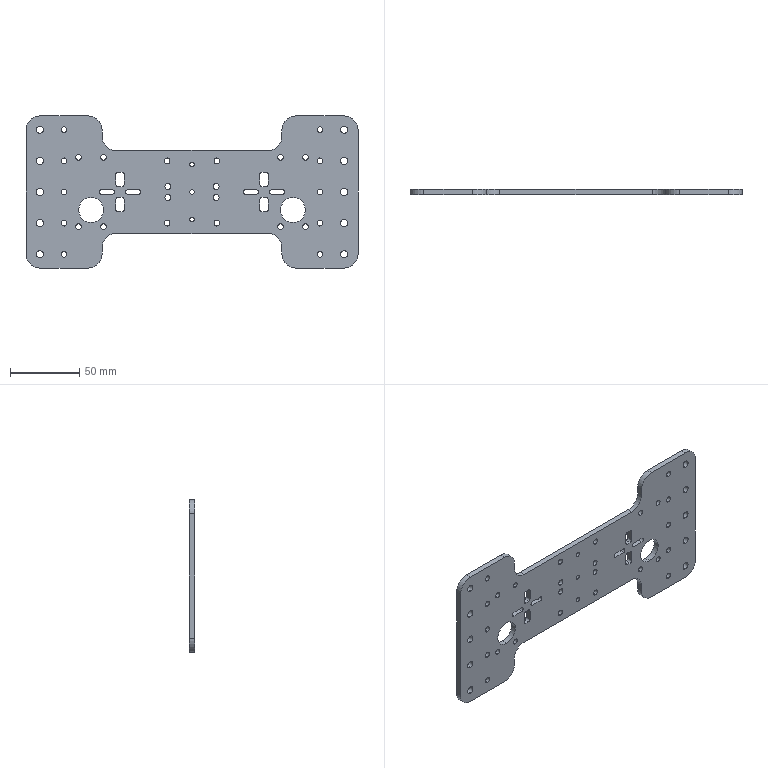Part | SolidWorks | features BaseBody 1 | 1 solid | 156 faces | box 240 x 4 x 110 mm | volume 73367 mm3 | cylinder 118 | plane 38 | commonest cylinder face diameters 4.2 x36 3.2 x30 4 x16 5.2 x16 20 x12 5.3 x4